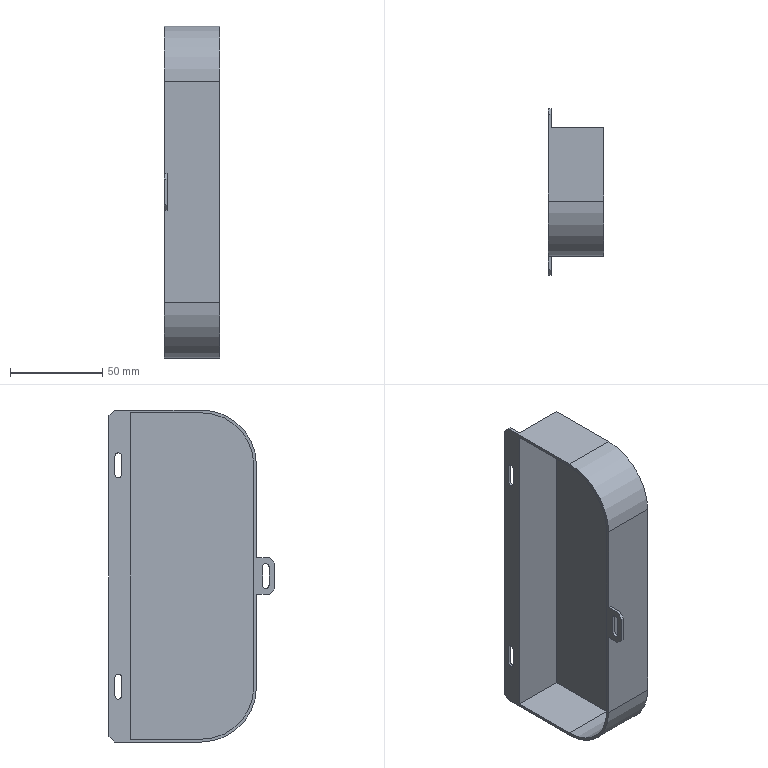Part | SolidWorks | features ICE 3, Chamfer 2, Extrusion 1, Shell 1 | 1 solid | 40 faces | box 30 x 90 x 180 mm | volume 41138 mm3 | plane 27 | cylinder 13 | commonest cylinder face diameters 3.5 x9 57 x2 60 x2
STEP:
#1=CARTESIAN_POINT('',(0.,-67.339,-42.431));
#2=VERTEX_POINT('',#1);
#3=CARTESIAN_POINT('',(0.,-65.589,-40.681));
#4=VERTEX_POINT('',#3);
#5=CARTESIAN_POINT('',(0.,-67.339,-40.681));
#6=DIRECTION('',(1.,0.,0.));
#7=DIRECTION('',(0.,0.,-1.));
#8=AXIS2_PLACEMENT_3D('',#5,#6,#7);
#9=CIRCLE('',#8,1.75);
#10=EDGE_CURVE('',#2,#4,#9,.T.);
#11=ORIENTED_EDGE('',*,*,#10,.F.);
#12=CARTESIAN_POINT('',(1.5,-67.339,-42.431));
#13=VERTEX_POINT('',#12);
#14=CARTESIAN_POINT('',(0.,-67.339,-42.431));
#15=DIRECTION('',(1.,0.,0.));
#16=VECTOR('',#15,1000.);
#17=LINE('',#14,#16);
#18=EDGE_CURVE('',#2,#13,#17,.T.);
#19=ORIENTED_EDGE('',*,*,#18,.T.);
#20=CARTESIAN_POINT('',(1.5,-65.589,-40.681));
#21=VERTEX_POINT('',#20);
#22=CARTESIAN_POINT('',(1.5,-67.339,-40.681));
#23=DIRECTION('',(1.,0.,0.));
#24=DIRECTION('',(0.,0.,-1.));
#25=AXIS2_PLACEMENT_3D('',#22,#23,#24);
#26=CIRCLE('',#25,1.75);
#27=EDGE_CURVE('',#13,#21,#26,.T.);
#28=ORIENTED_EDGE('',*,*,#27,.T.);
#29=CARTESIAN_POINT('',(0.,-65.589,-40.681));
#30=DIRECTION('',(1.,0.,0.));
#31=VECTOR('',#30,1000.);
#32=LINE('',#29,#31);
#33=EDGE_CURVE('',#4,#21,#32,.T.);
#34=ORIENTED_EDGE('',*,*,#33,.F.);
#35=EDGE_LOOP('',(#11,#19,#28,#34));
#36=FACE_OUTER_BOUND('',#35,.T.);
#37=CARTESIAN_POINT('',(0.,-67.339,-40.681));
#38=DIRECTION('',(1.,0.,0.));
#39=DIRECTION('',(0.,0.,-1.));
#40=AXIS2_PLACEMENT_3D('',#37,#38,#39);
#41=CYLINDRICAL_SURFACE('',#40,1.75);
#42=ADVANCED_FACE('',(#36),#41,.F.);
#43=CARTESIAN_POINT('',(0.,12.661,-102.431));
#44=VERTEX_POINT('',#43);
#45=CARTESIAN_POINT('',(0.,14.411,-100.681));
#46=VERTEX_POINT('',#45);
#47=CARTESIAN_POINT('',(0.,12.661,-100.681));
#48=DIRECTION('',(1.,0.,0.));
#49=DIRECTION('',(0.,0.,-1.));
#50=AXIS2_PLACEMENT_3D('',#47,#48,#49);
#51=CIRCLE('',#50,1.75);
#52=EDGE_CURVE('',#44,#46,#51,.T.);
#53=ORIENTED_EDGE('',*,*,#52,.F.);
#54=CARTESIAN_POINT('',(1.5,12.661,-102.431));
#55=VERTEX_POINT('',#54);
#56=CARTESIAN_POINT('',(0.,12.661,-102.431));
#57=DIRECTION('',(1.,0.,0.));
#58=VECTOR('',#57,1000.);
#59=LINE('',#56,#58);
#60=EDGE_CURVE('',#44,#55,#59,.T.);
#61=ORIENTED_EDGE('',*,*,#60,.T.);
#62=CARTESIAN_POINT('',(1.5,14.411,-100.681));
#63=VERTEX_POINT('',#62);
#64=CARTESIAN_POINT('',(1.5,12.661,-100.681));
#65=DIRECTION('',(1.,0.,0.));
#66=DIRECTION('',(0.,0.,-1.));
#67=AXIS2_PLACEMENT_3D('',#64,#65,#66);
#68=CIRCLE('',#67,1.75);
#69=EDGE_CURVE('',#55,#63,#68,.T.);
#70=ORIENTED_EDGE('',*,*,#69,.T.);
#71=CARTESIAN_POINT('',(0.,14.411,-100.681));
#72=DIRECTION('',(1.,0.,0.));
#73=VECTOR('',#72,1000.);
#74=LINE('',#71,#73);
#75=EDGE_CURVE('',#46,#63,#74,.T.);
#76=ORIENTED_EDGE('',*,*,#75,.F.);
#77=EDGE_LOOP('',(#53,#61,#70,#76));
#78=FACE_OUTER_BOUND('',#77,.T.);
#79=CARTESIAN_POINT('',(0.,12.661,-100.681));
#80=DIRECTION('',(1.,0.,0.));
#81=DIRECTION('',(0.,0.,-1.));
#82=AXIS2_PLACEMENT_3D('',#79,#80,#81);
#83=CYLINDRICAL_SURFACE('',#82,1.75);
#84=ADVANCED_FACE('',(#78),#83,.F.);
#85=CARTESIAN_POINT('',(0.,12.661,17.569));
#86=VERTEX_POINT('',#85);
#87=CARTESIAN_POINT('',(0.,14.411,19.319));
#88=VERTEX_POINT('',#87);
#89=CARTESIAN_POINT('',(0.,12.661,19.319));
#90=DIRECTION('',(1.,0.,0.));
#91=DIRECTION('',(0.,0.,-1.));
#92=AXIS2_PLACEMENT_3D('',#89,#90,#91);
#93=CIRCLE('',#92,1.75);
#94=EDGE_CURVE('',#86,#88,#93,.T.);
#95=ORIENTED_EDGE('',*,*,#94,.F.);
#96=CARTESIAN_POINT('',(1.5,12.661,17.569));
#97=VERTEX_POINT('',#96);
#98=CARTESIAN_POINT('',(0.,12.661,17.569));
#99=DIRECTION('',(1.,0.,0.));
#100=VECTOR('',#99,1000.);
#101=LINE('',#98,#100);
#102=EDGE_CURVE('',#86,#97,#101,.T.);
#103=ORIENTED_EDGE('',*,*,#102,.T.);
#104=CARTESIAN_POINT('',(1.5,14.411,19.319));
#105=VERTEX_POINT('',#104);
#106=CARTESIAN_POINT('',(1.5,12.661,19.319));
#107=DIRECTION('',(1.,0.,0.));
#108=DIRECTION('',(0.,0.,-1.));
#109=AXIS2_PLACEMENT_3D('',#106,#107,#108);
#110=CIRCLE('',#109,1.75);
#111=EDGE_CURVE('',#97,#105,#110,.T.);
#112=ORIENTED_EDGE('',*,*,#111,.T.);
#113=CARTESIAN_POINT('',(0.,14.411,19.319));
#114=DIRECTION('',(1.,0.,0.));
#115=VECTOR('',#114,1000.);
#116=LINE('',#113,#115);
#117=EDGE_CURVE('',#88,#105,#116,.T.);
#118=ORIENTED_EDGE('',*,*,#117,.F.);
#119=EDGE_LOOP('',(#95,#103,#112,#118));
#120=FACE_OUTER_BOUND('',#119,.T.);
#121=CARTESIAN_POINT('',(0.,12.661,19.319));
#122=DIRECTION('',(1.,0.,0.));
#123=DIRECTION('',(0.,0.,-1.));
#124=AXIS2_PLACEMENT_3D('',#121,#122,#123);
#125=CYLINDRICAL_SURFACE('',#124,1.75);
#126=ADVANCED_FACE('',(#120),#125,.F.);
#127=CARTESIAN_POINT('',(0.,-62.339,-45.681));
#128=VERTEX_POINT('',#127);
#129=CARTESIAN_POINT('',(1.5,-62.339,-45.681));
#130=VERTEX_POINT('',#129);
#131=CARTESIAN_POINT('',(0.,-62.339,-45.681));
#132=DIRECTION('',(1.,0.,0.));
#133=VECTOR('',#132,1000.);
#134=LINE('',#131,#133);
#135=EDGE_CURVE('',#128,#130,#134,.T.);
#136=ORIENTED_EDGE('',*,*,#135,.F.);
#137=CARTESIAN_POINT('',(0.,-62.339,-95.681));
#138=VERTEX_POINT('',#137);
#139=CARTESIAN_POINT('',(0.,-62.339,24.319));
#140=DIRECTION('',(0.,0.,-1.));
#141=VECTOR('',#140,1000.);
#142=LINE('',#139,#141);
#143=EDGE_CURVE('',#128,#138,#142,.T.);
#144=ORIENTED_EDGE('',*,*,#143,.T.);
#145=CARTESIAN_POINT('',(30.,-62.339,-95.681));
#146=VERTEX_POINT('',#145);
#147=CARTESIAN_POINT('',(30.,-62.339,-95.681));
#148=DIRECTION('',(-1.,0.,0.));
#149=VECTOR('',#148,1000.);
#150=LINE('',#147,#149);
#151=EDGE_CURVE('',#146,#138,#150,.T.);
#152=ORIENTED_EDGE('',*,*,#151,.F.);
#153=CARTESIAN_POINT('',(30.,-62.339,24.319));
#154=VERTEX_POINT('',#153);
#155=CARTESIAN_POINT('',(30.,-62.339,24.319));
#156=DIRECTION('',(0.,0.,-1.));
#157=VECTOR('',#156,1000.);
#158=LINE('',#155,#157);
#159=EDGE_CURVE('',#154,#146,#158,.T.);
#160=ORIENTED_EDGE('',*,*,#159,.F.);
#161=CARTESIAN_POINT('',(0.,-62.339,24.319));
#162=VERTEX_POINT('',#161);
#163=CARTESIAN_POINT('',(30.,-62.339,24.319));
#164=DIRECTION('',(-1.,0.,0.));
#165=VECTOR('',#164,1000.);
#166=LINE('',#163,#165);
#167=EDGE_CURVE('',#154,#162,#166,.T.);
#168=ORIENTED_EDGE('',*,*,#167,.T.);
#169=CARTESIAN_POINT('',(0.,-62.339,-25.681));
#170=VERTEX_POINT('',#169);
#171=CARTESIAN_POINT('',(0.,-62.339,24.319));
#172=DIRECTION('',(0.,0.,-1.));
#173=VECTOR('',#172,1000.);
#174=LINE('',#171,#173);
#175=EDGE_CURVE('',#162,#170,#174,.T.);
#176=ORIENTED_EDGE('',*,*,#175,.T.);
#177=CARTESIAN_POINT('',(1.5,-62.339,-25.681));
#178=VERTEX_POINT('',#177);
#179=CARTESIAN_POINT('',(0.,-62.339,-25.681));
#180=DIRECTION('',(-1.,0.,0.));
#181=VECTOR('',#180,1000.);
#182=LINE('',#179,#181);
#183=EDGE_CURVE('',#178,#170,#182,.T.);
#184=ORIENTED_EDGE('',*,*,#183,.F.);
#185=CARTESIAN_POINT('',(1.5,-62.339,-25.681));
#186=DIRECTION('',(0.,0.,1.));
#187=VECTOR('',#186,1000.);
#188=LINE('',#185,#187);
#189=EDGE_CURVE('',#130,#178,#188,.T.);
#190=ORIENTED_EDGE('',*,*,#189,.F.);
#191=EDGE_LOOP('',(#136,#144,#152,#160,#168,#176,#184,#190));
#192=FACE_OUTER_BOUND('',#191,.T.);
#193=CARTESIAN_POINT('',(30.,-62.339,24.319));
#194=DIRECTION('',(0.,1.,0.));
#195=DIRECTION('',(0.,0.,1.));
#196=AXIS2_PLACEMENT_3D('',#193,#194,#195);
#197=PLANE('',#196);
#198=ADVANCED_FACE('',(#192),#197,.F.);
#199=CARTESIAN_POINT('',(1.5,7.661,54.319));
#200=VERTEX_POINT('',#199);
#201=CARTESIAN_POINT('',(1.5,7.661,-125.681));
#202=VERTEX_POINT('',#201);
#203=CARTESIAN_POINT('',(1.5,7.661,54.319));
#204=DIRECTION('',(0.,0.,-1.));
#205=VECTOR('',#204,1000.);
#206=LINE('',#203,#205);
#207=EDGE_CURVE('',#200,#202,#206,.T.);
#208=ORIENTED_EDGE('',*,*,#207,.F.);
#209=CARTESIAN_POINT('',(30.,7.661,54.319));
#210=VERTEX_POINT('',#209);
#211=CARTESIAN_POINT('',(30.,7.661,54.319));
#212=DIRECTION('',(-1.,0.,0.));
#213=VECTOR('',#212,1000.);
#214=LINE('',#211,#213);
#215=EDGE_CURVE('',#210,#200,#214,.T.);
#216=ORIENTED_EDGE('',*,*,#215,.F.);
#217=CARTESIAN_POINT('',(30.,7.661,-125.681));
#218=VERTEX_POINT('',#217);
#219=CARTESIAN_POINT('',(30.,7.661,54.319));
#220=DIRECTION('',(0.,0.,1.));
#221=VECTOR('',#220,1000.);
#222=LINE('',#219,#221);
#223=EDGE_CURVE('',#218,#210,#222,.T.);
#224=ORIENTED_EDGE('',*,*,#223,.F.);
#225=CARTESIAN_POINT('',(30.,7.661,-125.681));
#226=DIRECTION('',(-1.,0.,0.));
#227=VECTOR('',#226,1000.);
#228=LINE('',#225,#227);
#229=EDGE_CURVE('',#218,#202,#228,.T.);
#230=ORIENTED_EDGE('',*,*,#229,.T.);
#231=EDGE_LOOP('',(#208,#216,#224,#230));
#232=FACE_OUTER_BOUND('',#231,.T.);
#233=CARTESIAN_POINT('',(30.,7.661,54.319));
#234=DIRECTION('',(0.,-1.,0.));
#235=DIRECTION('',(0.,0.,-1.));
#236=AXIS2_PLACEMENT_3D('',#233,#234,#235);
#237=PLANE('',#236);
#238=ADVANCED_FACE('',(#232),#237,.F.);
#239=CARTESIAN_POINT('',(0.,-65.589,-30.681));
#240=VERTEX_POINT('',#239);
#241=CARTESIAN_POINT('',(0.,-69.089,-30.681));
#242=VERTEX_POINT('',#241);
#243=CARTESIAN_POINT('',(0.,-67.339,-30.681));
#244=DIRECTION('',(1.,0.,0.));
#245=DIRECTION('',(0.,0.,-1.));
#246=AXIS2_PLACEMENT_3D('',#243,#244,#245);
#247=CIRCLE('',#246,1.75);
#248=EDGE_CURVE('',#240,#242,#247,.T.);
#249=ORIENTED_EDGE('',*,*,#248,.T.);
#250=CARTESIAN_POINT('',(0.,-69.089,-40.681));
#251=VERTEX_POINT('',#250);
#252=CARTESIAN_POINT('',(0.,-69.089,-30.681));
#253=DIRECTION('',(0.,0.,-1.));
#254=VECTOR('',#253,1000.);
#255=LINE('',#252,#254);
#256=EDGE_CURVE('',#242,#251,#255,.T.);
#257=ORIENTED_EDGE('',*,*,#256,.T.);
#258=CARTESIAN_POINT('',(0.,-67.339,-40.681));
#259=DIRECTION('',(1.,0.,0.));
#260=DIRECTION('',(0.,0.,-1.));
#261=AXIS2_PLACEMENT_3D('',#258,#259,#260);
#262=CIRCLE('',#261,1.75);
#263=EDGE_CURVE('',#251,#2,#262,.T.);
#264=ORIENTED_EDGE('',*,*,#263,.T.);
#265=ORIENTED_EDGE('',*,*,#10,.T.);
#266=CARTESIAN_POINT('',(0.,-65.589,-30.681));
#267=DIRECTION('',(0.,0.,1.));
#268=VECTOR('',#267,1000.);
#269=LINE('',#266,#268);
#270=EDGE_CURVE('',#4,#240,#269,.T.);
#271=ORIENTED_EDGE('',*,*,#270,.T.);
#272=EDGE_LOOP('',(#249,#257,#264,#265,#271));
#273=FACE_BOUND('',#272,.T.);
#274=CARTESIAN_POINT('',(0.,14.411,-90.681));
#275=VERTEX_POINT('',#274);
#276=CARTESIAN_POINT('',(0.,10.911,-90.681));
#277=VERTEX_POINT('',#276);
#278=CARTESIAN_POINT('',(0.,12.661,-90.681));
#279=DIRECTION('',(1.,0.,0.));
#280=DIRECTION('',(0.,0.,-1.));
#281=AXIS2_PLACEMENT_3D('',#278,#279,#280);
#282=CIRCLE('',#281,1.75);
#283=EDGE_CURVE('',#275,#277,#282,.T.);
#284=ORIENTED_EDGE('',*,*,#283,.T.);
#285=CARTESIAN_POINT('',(0.,10.911,-100.681));
#286=VERTEX_POINT('',#285);
#287=CARTESIAN_POINT('',(0.,10.911,-90.681));
#288=DIRECTION('',(0.,0.,-1.));
#289=VECTOR('',#288,1000.);
#290=LINE('',#287,#289);
#291=EDGE_CURVE('',#277,#286,#290,.T.);
#292=ORIENTED_EDGE('',*,*,#291,.T.);
#293=CARTESIAN_POINT('',(0.,12.661,-100.681));
#294=DIRECTION('',(1.,0.,0.));
#295=DIRECTION('',(0.,0.,-1.));
#296=AXIS2_PLACEMENT_3D('',#293,#294,#295);
#297=CIRCLE('',#296,1.75);
#298=EDGE_CURVE('',#286,#44,#297,.T.);
#299=ORIENTED_EDGE('',*,*,#298,.T.);
#300=ORIENTED_EDGE('',*,*,#52,.T.);
#301=CARTESIAN_POINT('',(0.,14.411,-90.681));
#302=DIRECTION('',(0.,0.,1.));
#303=VECTOR('',#302,1000.);
#304=LINE('',#301,#303);
#305=EDGE_CURVE('',#46,#275,#304,.T.);
#306=ORIENTED_EDGE('',*,*,#305,.T.);
#307=EDGE_LOOP('',(#284,#292,#299,#300,#306));
#308=FACE_BOUND('',#307,.T.);
#309=CARTESIAN_POINT('',(0.,14.411,29.319));
#310=VERTEX_POINT('',#309);
#311=CARTESIAN_POINT('',(0.,10.911,29.319));
#312=VERTEX_POINT('',#311);
#313=CARTESIAN_POINT('',(0.,12.661,29.319));
#314=DIRECTION('',(1.,0.,0.));
#315=DIRECTION('',(0.,0.,-1.));
#316=AXIS2_PLACEMENT_3D('',#313,#314,#315);
#317=CIRCLE('',#316,1.75);
#318=EDGE_CURVE('',#310,#312,#317,.T.);
#319=ORIENTED_EDGE('',*,*,#318,.T.);
#320=CARTESIAN_POINT('',(0.,10.911,19.319));
#321=VERTEX_POINT('',#320);
#322=CARTESIAN_POINT('',(0.,10.911,29.319));
#323=DIRECTION('',(0.,0.,-1.));
#324=VECTOR('',#323,1000.);
#325=LINE('',#322,#324);
#326=EDGE_CURVE('',#312,#321,#325,.T.);
#327=ORIENTED_EDGE('',*,*,#326,.T.);
#328=CARTESIAN_POINT('',(0.,12.661,19.319));
#329=DIRECTION('',(1.,0.,0.));
#330=DIRECTION('',(0.,0.,-1.));
#331=AXIS2_PLACEMENT_3D('',#328,#329,#330);
#332=CIRCLE('',#331,1.75);
#333=EDGE_CURVE('',#321,#86,#332,.T.);
#334=ORIENTED_EDGE('',*,*,#333,.T.);
#335=ORIENTED_EDGE('',*,*,#94,.T.);
#336=CARTESIAN_POINT('',(0.,14.411,29.319));
#337=DIRECTION('',(0.,0.,1.));
#338=VECTOR('',#337,1000.);
#339=LINE('',#336,#338);
#340=EDGE_CURVE('',#88,#310,#339,.T.);
#341=ORIENTED_EDGE('',*,*,#340,.T.);
#342=EDGE_LOOP('',(#319,#327,#334,#335,#341));
#343=FACE_BOUND('',#342,.T.);
#344=CARTESIAN_POINT('',(0.,-72.339,-28.681));
#345=VERTEX_POINT('',#344);
#346=CARTESIAN_POINT('',(0.,-72.339,-42.681));
#347=VERTEX_POINT('',#346);
#348=CARTESIAN_POINT('',(0.,-72.339,-25.681));
#349=DIRECTION('',(0.,0.,-1.));
#350=VECTOR('',#349,1000.);
#351=LINE('',#348,#350);
#352=EDGE_CURVE('',#345,#347,#351,.T.);
#353=ORIENTED_EDGE('',*,*,#352,.F.);
#354=CARTESIAN_POINT('',(0.,-69.339,-25.681));
#355=VERTEX_POINT('',#354);
#356=CARTESIAN_POINT('',(0.,-25.839,17.819));
#357=DIRECTION('',(0.,0.7071,0.7071));
#358=VECTOR('',#357,1000.);
#359=LINE('',#356,#358);
#360=EDGE_CURVE('',#345,#355,#359,.T.);
#361=ORIENTED_EDGE('',*,*,#360,.T.);
#362=CARTESIAN_POINT('',(0.,-72.339,-25.681));
#363=DIRECTION('',(0.,1.,0.));
#364=VECTOR('',#363,1000.);
#365=LINE('',#362,#364);
#366=EDGE_CURVE('',#355,#170,#365,.T.);
#367=ORIENTED_EDGE('',*,*,#366,.T.);
#368=ORIENTED_EDGE('',*,*,#175,.F.);
#369=CARTESIAN_POINT('',(0.,-32.339,54.319));
#370=VERTEX_POINT('',#369);
#371=CARTESIAN_POINT('',(0.,-32.339,24.319));
#372=DIRECTION('',(1.,0.,0.));
#373=DIRECTION('',(0.,0.,1.));
#374=AXIS2_PLACEMENT_3D('',#371,#372,#373);
#375=CIRCLE('',#374,30.);
#376=EDGE_CURVE('',#370,#162,#375,.T.);
#377=ORIENTED_EDGE('',*,*,#376,.F.);
#378=CARTESIAN_POINT('',(0.,14.661,54.319));
#379=VERTEX_POINT('',#378);
#380=CARTESIAN_POINT('',(0.,7.661,54.319));
#381=DIRECTION('',(0.,-1.,0.));
#382=VECTOR('',#381,1000.);
#383=LINE('',#380,#382);
#384=EDGE_CURVE('',#379,#370,#383,.T.);
#385=ORIENTED_EDGE('',*,*,#384,.F.);
#386=CARTESIAN_POINT('',(0.,17.661,51.319));
#387=VERTEX_POINT('',#386);
#388=CARTESIAN_POINT('',(0.,6.161,62.819));
#389=DIRECTION('',(0.,0.7071,-0.7071));
#390=VECTOR('',#389,1000.);
#391=LINE('',#388,#390);
#392=EDGE_CURVE('',#379,#387,#391,.T.);
#393=ORIENTED_EDGE('',*,*,#392,.T.);
#394=CARTESIAN_POINT('',(0.,17.661,-122.681));
#395=VERTEX_POINT('',#394);
#396=CARTESIAN_POINT('',(0.,17.661,54.319));
#397=DIRECTION('',(0.,0.,1.));
#398=VECTOR('',#397,1000.);
#399=LINE('',#396,#398);
#400=EDGE_CURVE('',#395,#387,#399,.T.);
#401=ORIENTED_EDGE('',*,*,#400,.F.);
#402=CARTESIAN_POINT('',(0.,14.661,-125.681));
#403=VERTEX_POINT('',#402);
#404=CARTESIAN_POINT('',(0.,66.161,-74.181));
#405=DIRECTION('',(0.,-0.7071,-0.7071));
#406=VECTOR('',#405,1000.);
#407=LINE('',#404,#406);
#408=EDGE_CURVE('',#395,#403,#407,.T.);
#409=ORIENTED_EDGE('',*,*,#408,.T.);
#410=CARTESIAN_POINT('',(0.,-32.339,-125.681));
#411=VERTEX_POINT('',#410);
#412=CARTESIAN_POINT('',(0.,7.661,-125.681));
#413=DIRECTION('',(0.,1.,0.));
#414=VECTOR('',#413,1000.);
#415=LINE('',#412,#414);
#416=EDGE_CURVE('',#411,#403,#415,.T.);
#417=ORIENTED_EDGE('',*,*,#416,.F.);
#418=CARTESIAN_POINT('',(0.,-32.339,-95.681));
#419=DIRECTION('',(1.,0.,0.));
#420=DIRECTION('',(0.,0.,-1.));
#421=AXIS2_PLACEMENT_3D('',#418,#419,#420);
#422=CIRCLE('',#421,30.);
#423=EDGE_CURVE('',#138,#411,#422,.T.);
#424=ORIENTED_EDGE('',*,*,#423,.F.);
#425=ORIENTED_EDGE('',*,*,#143,.F.);
#426=CARTESIAN_POINT('',(0.,-69.339,-45.681));
#427=VERTEX_POINT('',#426);
#428=CARTESIAN_POINT('',(0.,-72.339,-45.681));
#429=DIRECTION('',(0.,1.,0.));
#430=VECTOR('',#429,1000.);
#431=LINE('',#428,#430);
#432=EDGE_CURVE('',#427,#128,#431,.T.);
#433=ORIENTED_EDGE('',*,*,#432,.F.);
#434=CARTESIAN_POINT('',(0.,-85.839,-29.181));
#435=DIRECTION('',(0.,-0.7071,0.7071));
#436=VECTOR('',#435,1000.);
#437=LINE('',#434,#436);
#438=EDGE_CURVE('',#427,#347,#437,.T.);
#439=ORIENTED_EDGE('',*,*,#438,.T.);
#440=EDGE_LOOP('',(#353,#361,#367,#368,#377,#385,#393,#401,#409,#417,#424,#425,#433,#439));
#441=FACE_OUTER_BOUND('',#440,.T.);
#442=CARTESIAN_POINT('',(0.,6.161,-124.181));
#443=VERTEX_POINT('',#442);
#444=CARTESIAN_POINT('',(0.,6.161,52.819));
#445=VERTEX_POINT('',#444);
#446=CARTESIAN_POINT('',(0.,6.161,24.319));
#447=DIRECTION('',(0.,0.,1.));
#448=VECTOR('',#447,1000.);
#449=LINE('',#446,#448);
#450=EDGE_CURVE('',#443,#445,#449,.T.);
#451=ORIENTED_EDGE('',*,*,#450,.T.);
#452=CARTESIAN_POINT('',(0.,-32.339,52.819));
#453=VERTEX_POINT('',#452);
#454=CARTESIAN_POINT('',(0.,-32.339,52.819));
#455=DIRECTION('',(0.,-1.,0.));
#456=VECTOR('',#455,1000.);
#457=LINE('',#454,#456);
#458=EDGE_CURVE('',#445,#453,#457,.T.);
#459=ORIENTED_EDGE('',*,*,#458,.T.);
#460=CARTESIAN_POINT('',(0.,-60.839,24.319));
#461=VERTEX_POINT('',#460);
#462=CARTESIAN_POINT('',(0.,-32.339,24.319));
#463=DIRECTION('',(1.,0.,0.));
#464=DIRECTION('',(0.,0.,1.));
#465=AXIS2_PLACEMENT_3D('',#462,#463,#464);
#466=CIRCLE('',#465,28.5);
#467=EDGE_CURVE('',#453,#461,#466,.T.);
#468=ORIENTED_EDGE('',*,*,#467,.T.);
#469=CARTESIAN_POINT('',(0.,-60.839,-95.681));
#470=VERTEX_POINT('',#469);
#471=CARTESIAN_POINT('',(0.,-60.839,24.319));
#472=DIRECTION('',(0.,0.,-1.));
#473=VECTOR('',#472,1000.);
#474=LINE('',#471,#473);
#475=EDGE_CURVE('',#461,#470,#474,.T.);
#476=ORIENTED_EDGE('',*,*,#475,.T.);
#477=CARTESIAN_POINT('',(0.,-32.339,-124.181));
#478=VERTEX_POINT('',#477);
#479=CARTESIAN_POINT('',(0.,-32.339,-95.681));
#480=DIRECTION('',(1.,0.,0.));
#481=DIRECTION('',(0.,0.,1.));
#482=AXIS2_PLACEMENT_3D('',#479,#480,#481);
#483=CIRCLE('',#482,28.5);
#484=EDGE_CURVE('',#470,#478,#483,.T.);
#485=ORIENTED_EDGE('',*,*,#484,.T.);
#486=CARTESIAN_POINT('',(0.,-32.339,-124.181));
#487=DIRECTION('',(0.,1.,0.));
#488=VECTOR('',#487,1000.);
#489=LINE('',#486,#488);
#490=EDGE_CURVE('',#478,#443,#489,.T.);
#491=ORIENTED_EDGE('',*,*,#490,.T.);
#492=EDGE_LOOP('',(#451,#459,#468,#476,#485,#491));
#493=FACE_BOUND('',#492,.T.);
#494=CARTESIAN_POINT('',(0.,-32.339,24.319));
#495=DIRECTION('',(-1.,0.,0.));
#496=DIRECTION('',(0.,0.,1.));
#497=AXIS2_PLACEMENT_3D('',#494,#495,#496);
#498=PLANE('',#497);
#499=ADVANCED_FACE('',(#273,#308,#343,#441,#493),#498,.T.);
#500=CARTESIAN_POINT('',(1.5,14.661,54.319));
#501=VERTEX_POINT('',#500);
#502=CARTESIAN_POINT('',(1.5,17.661,54.319));
#503=DIRECTION('',(0.,-1.,0.));
#504=VECTOR('',#503,1000.);
#505=LINE('',#502,#504);
#506=EDGE_CURVE('',#501,#200,#505,.T.);
#507=ORIENTED_EDGE('',*,*,#506,.F.);
#508=CARTESIAN_POINT('',(30.,14.661,54.319));
#509=DIRECTION('',(-1.,0.,0.));
#510=VECTOR('',#509,1000.);
#511=LINE('',#508,#510);
#512=EDGE_CURVE('',#501,#379,#511,.T.);
#513=ORIENTED_EDGE('',*,*,#512,.T.);
#514=ORIENTED_EDGE('',*,*,#384,.T.);
#515=CARTESIAN_POINT('',(30.,-32.339,54.319));
#516=VERTEX_POINT('',#515);
#517=CARTESIAN_POINT('',(30.,-32.339,54.319));
#518=DIRECTION('',(-1.,0.,0.));
#519=VECTOR('',#518,1000.);
#520=LINE('',#517,#519);
#521=EDGE_CURVE('',#516,#370,#520,.T.);
#522=ORIENTED_EDGE('',*,*,#521,.F.);
#523=CARTESIAN_POINT('',(30.,7.661,54.319));
#524=DIRECTION('',(0.,-1.,0.));
#525=VECTOR('',#524,1000.);
#526=LINE('',#523,#525);
#527=EDGE_CURVE('',#210,#516,#526,.T.);
#528=ORIENTED_EDGE('',*,*,#527,.F.);
#529=ORIENTED_EDGE('',*,*,#215,.T.);
#530=EDGE_LOOP('',(#507,#513,#514,#522,#528,#529));
#531=FACE_OUTER_BOUND('',#530,.T.);
#532=CARTESIAN_POINT('',(30.,7.661,54.319));
#533=DIRECTION('',(0.,0.,-1.));
#534=DIRECTION('',(0.,1.,0.));
#535=AXIS2_PLACEMENT_3D('',#532,#533,#534);
#536=PLANE('',#535);
#537=ADVANCED_FACE('',(#531),#536,.F.);
#538=ORIENTED_EDGE('',*,*,#376,.T.);
#539=ORIENTED_EDGE('',*,*,#167,.F.);
#540=CARTESIAN_POINT('',(30.,-32.339,24.319));
#541=DIRECTION('',(1.,0.,0.));
#542=DIRECTION('',(0.,0.,1.));
#543=AXIS2_PLACEMENT_3D('',#540,#541,#542);
#544=CIRCLE('',#543,30.);
#545=EDGE_CURVE('',#516,#154,#544,.T.);
#546=ORIENTED_EDGE('',*,*,#545,.F.);
#547=ORIENTED_EDGE('',*,*,#521,.T.);
#548=EDGE_LOOP('',(#538,#539,#546,#547));
#549=FACE_OUTER_BOUND('',#548,.T.);
#550=CARTESIAN_POINT('',(30.,-32.339,24.319));
#551=DIRECTION('',(-1.,0.,0.));
#552=DIRECTION('',(0.,0.,1.));
#553=AXIS2_PLACEMENT_3D('',#550,#551,#552);
#554=CYLINDRICAL_SURFACE('',#553,30.);
#555=ADVANCED_FACE('',(#549),#554,.T.);
#556=ORIENTED_EDGE('',*,*,#423,.T.);
#557=CARTESIAN_POINT('',(30.,-32.339,-125.681));
#558=VERTEX_POINT('',#557);
#559=CARTESIAN_POINT('',(30.,-32.339,-125.681));
#560=DIRECTION('',(-1.,0.,0.));
#561=VECTOR('',#560,1000.);
#562=LINE('',#559,#561);
#563=EDGE_CURVE('',#558,#411,#562,.T.);
#564=ORIENTED_EDGE('',*,*,#563,.F.);
#565=CARTESIAN_POINT('',(30.,-32.339,-95.681));
#566=DIRECTION('',(1.,0.,0.));
#567=DIRECTION('',(0.,0.,-1.));
#568=AXIS2_PLACEMENT_3D('',#565,#566,#567);
#569=CIRCLE('',#568,30.);
#570=EDGE_CURVE('',#146,#558,#569,.T.);
#571=ORIENTED_EDGE('',*,*,#570,.F.);
#572=ORIENTED_EDGE('',*,*,#151,.T.);
#573=EDGE_LOOP('',(#556,#564,#571,#572));
#574=FACE_OUTER_BOUND('',#573,.T.);
#575=CARTESIAN_POINT('',(30.,-32.339,-95.681));
#576=DIRECTION('',(-1.,0.,0.));
#577=DIRECTION('',(0.,0.,1.));
#578=AXIS2_PLACEMENT_3D('',#575,#576,#577);
#579=CYLINDRICAL_SURFACE('',#578,30.);
#580=ADVANCED_FACE('',(#574),#579,.T.);
#581=ORIENTED_EDGE('',*,*,#416,.T.);
#582=CARTESIAN_POINT('',(1.5,14.661,-125.681));
#583=VERTEX_POINT('',#582);
#584=CARTESIAN_POINT('',(30.,14.661,-125.681));
#585=DIRECTION('',(1.,0.,0.));
#586=VECTOR('',#585,1000.);
#587=LINE('',#584,#586);
#588=EDGE_CURVE('',#403,#583,#587,.T.);
#589=ORIENTED_EDGE('',*,*,#588,.T.);
#590=CARTESIAN_POINT('',(1.5,17.661,-125.681));
#591=DIRECTION('',(0.,-1.,0.));
#592=VECTOR('',#591,1000.);
#593=LINE('',#590,#592);
#594=EDGE_CURVE('',#583,#202,#593,.T.);
#595=ORIENTED_EDGE('',*,*,#594,.T.);
#596=ORIENTED_EDGE('',*,*,#229,.F.);
#597=CARTESIAN_POINT('',(30.,7.661,-125.681));
#598=DIRECTION('',(0.,1.,0.));
#599=VECTOR('',#598,1000.);
#600=LINE('',#597,#599);
#601=EDGE_CURVE('',#558,#218,#600,.T.);
#602=ORIENTED_EDGE('',*,*,#601,.F.);
#603=ORIENTED_EDGE('',*,*,#563,.T.);
#604=EDGE_LOOP('',(#581,#589,#595,#596,#602,#603));
#605=FACE_OUTER_BOUND('',#604,.T.);
#606=CARTESIAN_POINT('',(30.,7.661,-125.681));
#607=DIRECTION('',(0.,0.,1.));
#608=DIRECTION('',(1.,0.,0.));
#609=AXIS2_PLACEMENT_3D('',#606,#607,#608);
#610=PLANE('',#609);
#611=ADVANCED_FACE('',(#605),#610,.F.);
#612=ORIENTED_EDGE('',*,*,#527,.T.);
#613=ORIENTED_EDGE('',*,*,#545,.T.);
#614=ORIENTED_EDGE('',*,*,#159,.T.);
#615=ORIENTED_EDGE('',*,*,#570,.T.);
#616=ORIENTED_EDGE('',*,*,#601,.T.);
#617=ORIENTED_EDGE('',*,*,#223,.T.);
#618=EDGE_LOOP('',(#612,#613,#614,#615,#616,#617));
#619=FACE_OUTER_BOUND('',#618,.T.);
#620=CARTESIAN_POINT('',(30.,-32.339,24.319));
#621=DIRECTION('',(-1.,0.,0.));
#622=DIRECTION('',(0.,0.,1.));
#623=AXIS2_PLACEMENT_3D('',#620,#621,#622);
#624=PLANE('',#623);
#625=ADVANCED_FACE('',(#619),#624,.F.);
#626=ORIENTED_EDGE('',*,*,#458,.F.);
#627=CARTESIAN_POINT('',(28.5,6.161,52.819));
#628=VERTEX_POINT('',#627);
#629=CARTESIAN_POINT('',(30.,6.161,52.819));
#630=DIRECTION('',(-1.,0.,0.));
#631=VECTOR('',#630,1000.);
#632=LINE('',#629,#631);
#633=EDGE_CURVE('',#628,#445,#632,.T.);
#634=ORIENTED_EDGE('',*,*,#633,.F.);
#635=CARTESIAN_POINT('',(28.5,-32.339,52.819));
#636=VERTEX_POINT('',#635);
#637=CARTESIAN_POINT('',(28.5,-32.339,52.819));
#638=DIRECTION('',(0.,-1.,0.));
#639=VECTOR('',#638,1000.);
#640=LINE('',#637,#639);
#641=EDGE_CURVE('',#628,#636,#640,.T.);
#642=ORIENTED_EDGE('',*,*,#641,.T.);
#643=CARTESIAN_POINT('',(30.,-32.339,52.819));
#644=DIRECTION('',(-1.,0.,0.));
#645=VECTOR('',#644,1000.);
#646=LINE('',#643,#645);
#647=EDGE_CURVE('',#636,#453,#646,.T.);
#648=ORIENTED_EDGE('',*,*,#647,.T.);
#649=EDGE_LOOP('',(#626,#634,#642,#648));
#650=FACE_OUTER_BOUND('',#649,.T.);
#651=CARTESIAN_POINT('',(30.,7.661,52.819));
#652=DIRECTION('',(0.,0.,-1.));
#653=DIRECTION('',(0.,1.,0.));
#654=AXIS2_PLACEMENT_3D('',#651,#652,#653);
#655=PLANE('',#654);
#656=ADVANCED_FACE('',(#650),#655,.T.);
#657=ORIENTED_EDGE('',*,*,#467,.F.);
#658=ORIENTED_EDGE('',*,*,#647,.F.);
#659=CARTESIAN_POINT('',(28.5,-60.839,24.319));
#660=VERTEX_POINT('',#659);
#661=CARTESIAN_POINT('',(28.5,-32.339,24.319));
#662=DIRECTION('',(1.,0.,0.));
#663=DIRECTION('',(0.,0.,1.));
#664=AXIS2_PLACEMENT_3D('',#661,#662,#663);
#665=CIRCLE('',#664,28.5);
#666=EDGE_CURVE('',#636,#660,#665,.T.);
#667=ORIENTED_EDGE('',*,*,#666,.T.);
#668=CARTESIAN_POINT('',(30.,-60.839,24.319));
#669=DIRECTION('',(-1.,0.,0.));
#670=VECTOR('',#669,1000.);
#671=LINE('',#668,#670);
#672=EDGE_CURVE('',#660,#461,#671,.T.);
#673=ORIENTED_EDGE('',*,*,#672,.T.);
#674=EDGE_LOOP('',(#657,#658,#667,#673));
#675=FACE_OUTER_BOUND('',#674,.T.);
#676=CARTESIAN_POINT('',(30.,-32.339,24.319));
#677=DIRECTION('',(-1.,0.,0.));
#678=DIRECTION('',(0.,0.,1.));
#679=AXIS2_PLACEMENT_3D('',#676,#677,#678);
#680=CYLINDRICAL_SURFACE('',#679,28.5);
#681=ADVANCED_FACE('',(#675),#680,.F.);
#682=ORIENTED_EDGE('',*,*,#475,.F.);
#683=ORIENTED_EDGE('',*,*,#672,.F.);
#684=CARTESIAN_POINT('',(28.5,-60.839,-95.681));
#685=VERTEX_POINT('',#684);
#686=CARTESIAN_POINT('',(28.5,-60.839,24.319));
#687=DIRECTION('',(0.,0.,-1.));
#688=VECTOR('',#687,1000.);
#689=LINE('',#686,#688);
#690=EDGE_CURVE('',#660,#685,#689,.T.);
#691=ORIENTED_EDGE('',*,*,#690,.T.);
#692=CARTESIAN_POINT('',(30.,-60.839,-95.681));
#693=DIRECTION('',(-1.,0.,0.));
#694=VECTOR('',#693,1000.);
#695=LINE('',#692,#694);
#696=EDGE_CURVE('',#685,#470,#695,.T.);
#697=ORIENTED_EDGE('',*,*,#696,.T.);
#698=EDGE_LOOP('',(#682,#683,#691,#697));
#699=FACE_OUTER_BOUND('',#698,.T.);
#700=CARTESIAN_POINT('',(30.,-60.839,24.319));
#701=DIRECTION('',(0.,1.,0.));
#702=DIRECTION('',(0.,0.,1.));
#703=AXIS2_PLACEMENT_3D('',#700,#701,#702);
#704=PLANE('',#703);
#705=ADVANCED_FACE('',(#699),#704,.T.);
#706=ORIENTED_EDGE('',*,*,#484,.F.);
#707=ORIENTED_EDGE('',*,*,#696,.F.);
#708=CARTESIAN_POINT('',(28.5,-32.339,-124.181));
#709=VERTEX_POINT('',#708);
#710=CARTESIAN_POINT('',(28.5,-32.339,-95.681));
#711=DIRECTION('',(1.,0.,0.));
#712=DIRECTION('',(0.,0.,1.));
#713=AXIS2_PLACEMENT_3D('',#710,#711,#712);
#714=CIRCLE('',#713,28.5);
#715=EDGE_CURVE('',#685,#709,#714,.T.);
#716=ORIENTED_EDGE('',*,*,#715,.T.);
#717=CARTESIAN_POINT('',(30.,-32.339,-124.181));
#718=DIRECTION('',(-1.,0.,0.));
#719=VECTOR('',#718,1000.);
#720=LINE('',#717,#719);
#721=EDGE_CURVE('',#709,#478,#720,.T.);
#722=ORIENTED_EDGE('',*,*,#721,.T.);
#723=EDGE_LOOP('',(#706,#707,#716,#722));
#724=FACE_OUTER_BOUND('',#723,.T.);
#725=CARTESIAN_POINT('',(30.,-32.339,-95.681));
#726=DIRECTION('',(-1.,0.,0.));
#727=DIRECTION('',(0.,0.,1.));
#728=AXIS2_PLACEMENT_3D('',#725,#726,#727);
#729=CYLINDRICAL_SURFACE('',#728,28.5);
#730=ADVANCED_FACE('',(#724),#729,.F.);
#731=ORIENTED_EDGE('',*,*,#490,.F.);
#732=ORIENTED_EDGE('',*,*,#721,.F.);
#733=CARTESIAN_POINT('',(28.5,6.161,-124.181));
#734=VERTEX_POINT('',#733);
#735=CARTESIAN_POINT('',(28.5,-32.339,-124.181));
#736=DIRECTION('',(0.,1.,0.));
#737=VECTOR('',#736,1000.);
#738=LINE('',#735,#737);
#739=EDGE_CURVE('',#709,#734,#738,.T.);
#740=ORIENTED_EDGE('',*,*,#739,.T.);
#741=CARTESIAN_POINT('',(30.,6.161,-124.181));
#742=DIRECTION('',(-1.,0.,0.));
#743=VECTOR('',#742,1000.);
#744=LINE('',#741,#743);
#745=EDGE_CURVE('',#734,#443,#744,.T.);
#746=ORIENTED_EDGE('',*,*,#745,.T.);
#747=EDGE_LOOP('',(#731,#732,#740,#746));
#748=FACE_OUTER_BOUND('',#747,.T.);
#749=CARTESIAN_POINT('',(30.,7.661,-124.181));
#750=DIRECTION('',(0.,0.,1.));
#751=DIRECTION('',(1.,0.,0.));
#752=AXIS2_PLACEMENT_3D('',#749,#750,#751);
#753=PLANE('',#752);
#754=ADVANCED_FACE('',(#748),#753,.T.);
#755=ORIENTED_EDGE('',*,*,#450,.F.);
#756=ORIENTED_EDGE('',*,*,#745,.F.);
#757=CARTESIAN_POINT('',(28.5,6.161,24.319));
#758=DIRECTION('',(0.,0.,1.));
#759=VECTOR('',#758,1000.);
#760=LINE('',#757,#759);
#761=EDGE_CURVE('',#734,#628,#760,.T.);
#762=ORIENTED_EDGE('',*,*,#761,.T.);
#763=ORIENTED_EDGE('',*,*,#633,.T.);
#764=EDGE_LOOP('',(#755,#756,#762,#763));
#765=FACE_OUTER_BOUND('',#764,.T.);
#766=CARTESIAN_POINT('',(30.,6.161,54.319));
#767=DIRECTION('',(0.,-1.,0.));
#768=DIRECTION('',(0.,0.,-1.));
#769=AXIS2_PLACEMENT_3D('',#766,#767,#768);
#770=PLANE('',#769);
#771=ADVANCED_FACE('',(#765),#770,.T.);
#772=ORIENTED_EDGE('',*,*,#641,.F.);
#773=ORIENTED_EDGE('',*,*,#761,.F.);
#774=ORIENTED_EDGE('',*,*,#739,.F.);
#775=ORIENTED_EDGE('',*,*,#715,.F.);
#776=ORIENTED_EDGE('',*,*,#690,.F.);
#777=ORIENTED_EDGE('',*,*,#666,.F.);
#778=EDGE_LOOP('',(#772,#773,#774,#775,#776,#777));
#779=FACE_OUTER_BOUND('',#778,.T.);
#780=CARTESIAN_POINT('',(28.5,-32.339,24.319));
#781=DIRECTION('',(-1.,0.,0.));
#782=DIRECTION('',(0.,0.,1.));
#783=AXIS2_PLACEMENT_3D('',#780,#781,#782);
#784=PLANE('',#783);
#785=ADVANCED_FACE('',(#779),#784,.T.);
#786=CARTESIAN_POINT('',(1.5,10.911,-90.681));
#787=VERTEX_POINT('',#786);
#788=CARTESIAN_POINT('',(1.5,10.911,-100.681));
#789=VERTEX_POINT('',#788);
#790=CARTESIAN_POINT('',(1.5,10.911,-90.681));
#791=DIRECTION('',(0.,0.,-1.));
#792=VECTOR('',#791,1000.);
#793=LINE('',#790,#792);
#794=EDGE_CURVE('',#787,#789,#793,.T.);
#795=ORIENTED_EDGE('',*,*,#794,.F.);
#796=CARTESIAN_POINT('',(1.5,14.411,-90.681));
#797=VERTEX_POINT('',#796);
#798=CARTESIAN_POINT('',(1.5,12.661,-90.681));
#799=DIRECTION('',(1.,0.,0.));
#800=DIRECTION('',(0.,0.,-1.));
#801=AXIS2_PLACEMENT_3D('',#798,#799,#800);
#802=CIRCLE('',#801,1.75);
#803=EDGE_CURVE('',#797,#787,#802,.T.);
#804=ORIENTED_EDGE('',*,*,#803,.F.);
#805=CARTESIAN_POINT('',(1.5,14.411,-90.681));
#806=DIRECTION('',(0.,0.,1.));
#807=VECTOR('',#806,1000.);
#808=LINE('',#805,#807);
#809=EDGE_CURVE('',#63,#797,#808,.T.);
#810=ORIENTED_EDGE('',*,*,#809,.F.);
#811=ORIENTED_EDGE('',*,*,#69,.F.);
#812=CARTESIAN_POINT('',(1.5,12.661,-100.681));
#813=DIRECTION('',(1.,0.,0.));
#814=DIRECTION('',(0.,0.,-1.));
#815=AXIS2_PLACEMENT_3D('',#812,#813,#814);
#816=CIRCLE('',#815,1.75);
#817=EDGE_CURVE('',#789,#55,#816,.T.);
#818=ORIENTED_EDGE('',*,*,#817,.F.);
#819=EDGE_LOOP('',(#795,#804,#810,#811,#818));
#820=FACE_BOUND('',#819,.T.);
#821=CARTESIAN_POINT('',(1.5,10.911,29.319));
#822=VERTEX_POINT('',#821);
#823=CARTESIAN_POINT('',(1.5,10.911,19.319));
#824=VERTEX_POINT('',#823);
#825=CARTESIAN_POINT('',(1.5,10.911,29.319));
#826=DIRECTION('',(0.,0.,-1.));
#827=VECTOR('',#826,1000.);
#828=LINE('',#825,#827);
#829=EDGE_CURVE('',#822,#824,#828,.T.);
#830=ORIENTED_EDGE('',*,*,#829,.F.);
#831=CARTESIAN_POINT('',(1.5,14.411,29.319));
#832=VERTEX_POINT('',#831);
#833=CARTESIAN_POINT('',(1.5,12.661,29.319));
#834=DIRECTION('',(1.,0.,0.));
#835=DIRECTION('',(0.,0.,-1.));
#836=AXIS2_PLACEMENT_3D('',#833,#834,#835);
#837=CIRCLE('',#836,1.75);
#838=EDGE_CURVE('',#832,#822,#837,.T.);
#839=ORIENTED_EDGE('',*,*,#838,.F.);
#840=CARTESIAN_POINT('',(1.5,14.411,29.319));
#841=DIRECTION('',(0.,0.,1.));
#842=VECTOR('',#841,1000.);
#843=LINE('',#840,#842);
#844=EDGE_CURVE('',#105,#832,#843,.T.);
#845=ORIENTED_EDGE('',*,*,#844,.F.);
#846=ORIENTED_EDGE('',*,*,#111,.F.);
#847=CARTESIAN_POINT('',(1.5,12.661,19.319));
#848=DIRECTION('',(1.,0.,0.));
#849=DIRECTION('',(0.,0.,-1.));
#850=AXIS2_PLACEMENT_3D('',#847,#848,#849);
#851=CIRCLE('',#850,1.75);
#852=EDGE_CURVE('',#824,#97,#851,.T.);
#853=ORIENTED_EDGE('',*,*,#852,.F.);
#854=EDGE_LOOP('',(#830,#839,#845,#846,#853));
#855=FACE_BOUND('',#854,.T.);
#856=ORIENTED_EDGE('',*,*,#594,.F.);
#857=CARTESIAN_POINT('',(1.5,17.661,-122.681));
#858=VERTEX_POINT('',#857);
#859=CARTESIAN_POINT('',(1.5,17.661,-122.681));
#860=DIRECTION('',(0.,0.7071,0.7071));
#861=VECTOR('',#860,1000.);
#862=LINE('',#859,#861);
#863=EDGE_CURVE('',#583,#858,#862,.T.);
#864=ORIENTED_EDGE('',*,*,#863,.T.);
#865=CARTESIAN_POINT('',(1.5,17.661,51.319));
#866=VERTEX_POINT('',#865);
#867=CARTESIAN_POINT('',(1.5,17.661,54.319));
#868=DIRECTION('',(0.,0.,-1.));
#869=VECTOR('',#868,1000.);
#870=LINE('',#867,#869);
#871=EDGE_CURVE('',#866,#858,#870,.T.);
#872=ORIENTED_EDGE('',*,*,#871,.F.);
#873=CARTESIAN_POINT('',(1.5,17.661,51.319));
#874=DIRECTION('',(0.,-0.7071,0.7071));
#875=VECTOR('',#874,1000.);
#876=LINE('',#873,#875);
#877=EDGE_CURVE('',#866,#501,#876,.T.);
#878=ORIENTED_EDGE('',*,*,#877,.T.);
#879=ORIENTED_EDGE('',*,*,#506,.T.);
#880=ORIENTED_EDGE('',*,*,#207,.T.);
#881=EDGE_LOOP('',(#856,#864,#872,#878,#879,#880));
#882=FACE_OUTER_BOUND('',#881,.T.);
#883=CARTESIAN_POINT('',(1.5,17.661,54.319));
#884=DIRECTION('',(-1.,0.,0.));
#885=DIRECTION('',(0.,0.,1.));
#886=AXIS2_PLACEMENT_3D('',#883,#884,#885);
#887=PLANE('',#886);
#888=ADVANCED_FACE('',(#820,#855,#882),#887,.F.);
#889=ORIENTED_EDGE('',*,*,#871,.T.);
#890=CARTESIAN_POINT('',(0.,17.661,-122.681));
#891=DIRECTION('',(-1.,0.,0.));
#892=VECTOR('',#891,1000.);
#893=LINE('',#890,#892);
#894=EDGE_CURVE('',#858,#395,#893,.T.);
#895=ORIENTED_EDGE('',*,*,#894,.T.);
#896=ORIENTED_EDGE('',*,*,#400,.T.);
#897=CARTESIAN_POINT('',(0.,17.661,51.319));
#898=DIRECTION('',(1.,0.,0.));
#899=VECTOR('',#898,1000.);
#900=LINE('',#897,#899);
#901=EDGE_CURVE('',#387,#866,#900,.T.);
#902=ORIENTED_EDGE('',*,*,#901,.T.);
#903=EDGE_LOOP('',(#889,#895,#896,#902));
#904=FACE_OUTER_BOUND('',#903,.T.);
#905=CARTESIAN_POINT('',(0.,17.661,0.));
#906=DIRECTION('',(0.,-1.,0.));
#907=DIRECTION('',(0.,0.,-1.));
#908=AXIS2_PLACEMENT_3D('',#905,#906,#907);
#909=PLANE('',#908);
#910=ADVANCED_FACE('',(#904),#909,.F.);
#911=CARTESIAN_POINT('',(1.5,-69.339,-45.681));
#912=VERTEX_POINT('',#911);
#913=CARTESIAN_POINT('',(1.5,-72.339,-45.681));
#914=DIRECTION('',(0.,1.,0.));
#915=VECTOR('',#914,1000.);
#916=LINE('',#913,#915);
#917=EDGE_CURVE('',#912,#130,#916,.T.);
#918=ORIENTED_EDGE('',*,*,#917,.F.);
#919=CARTESIAN_POINT('',(0.,-69.339,-45.681));
#920=DIRECTION('',(-1.,0.,0.));
#921=VECTOR('',#920,1000.);
#922=LINE('',#919,#921);
#923=EDGE_CURVE('',#912,#427,#922,.T.);
#924=ORIENTED_EDGE('',*,*,#923,.T.);
#925=ORIENTED_EDGE('',*,*,#432,.T.);
#926=ORIENTED_EDGE('',*,*,#135,.T.);
#927=EDGE_LOOP('',(#918,#924,#925,#926));
#928=FACE_OUTER_BOUND('',#927,.T.);
#929=CARTESIAN_POINT('',(0.,-72.339,-45.681));
#930=DIRECTION('',(0.,0.,1.));
#931=DIRECTION('',(1.,0.,0.));
#932=AXIS2_PLACEMENT_3D('',#929,#930,#931);
#933=PLANE('',#932);
#934=ADVANCED_FACE('',(#928),#933,.F.);
#935=CARTESIAN_POINT('',(1.5,-69.089,-30.681));
#936=VERTEX_POINT('',#935);
#937=CARTESIAN_POINT('',(1.5,-69.089,-40.681));
#938=VERTEX_POINT('',#937);
#939=CARTESIAN_POINT('',(1.5,-69.089,-30.681));
#940=DIRECTION('',(0.,0.,-1.));
#941=VECTOR('',#940,1000.);
#942=LINE('',#939,#941);
#943=EDGE_CURVE('',#936,#938,#942,.T.);
#944=ORIENTED_EDGE('',*,*,#943,.F.);
#945=CARTESIAN_POINT('',(1.5,-65.589,-30.681));
#946=VERTEX_POINT('',#945);
#947=CARTESIAN_POINT('',(1.5,-67.339,-30.681));
#948=DIRECTION('',(1.,0.,0.));
#949=DIRECTION('',(0.,0.,-1.));
#950=AXIS2_PLACEMENT_3D('',#947,#948,#949);
#951=CIRCLE('',#950,1.75);
#952=EDGE_CURVE('',#946,#936,#951,.T.);
#953=ORIENTED_EDGE('',*,*,#952,.F.);
#954=CARTESIAN_POINT('',(1.5,-65.589,-30.681));
#955=DIRECTION('',(0.,0.,1.));
#956=VECTOR('',#955,1000.);
#957=LINE('',#954,#956);
#958=EDGE_CURVE('',#21,#946,#957,.T.);
#959=ORIENTED_EDGE('',*,*,#958,.F.);
#960=ORIENTED_EDGE('',*,*,#27,.F.);
#961=CARTESIAN_POINT('',(1.5,-67.339,-40.681));
#962=DIRECTION('',(1.,0.,0.));
#963=DIRECTION('',(0.,0.,-1.));
#964=AXIS2_PLACEMENT_3D('',#961,#962,#963);
#965=CIRCLE('',#964,1.75);
#966=EDGE_CURVE('',#938,#13,#965,.T.);
#967=ORIENTED_EDGE('',*,*,#966,.F.);
#968=EDGE_LOOP('',(#944,#953,#959,#960,#967));
#969=FACE_BOUND('',#968,.T.);
#970=CARTESIAN_POINT('',(1.5,-69.339,-25.681));
#971=VERTEX_POINT('',#970);
#972=CARTESIAN_POINT('',(1.5,-72.339,-25.681));
#973=DIRECTION('',(0.,1.,0.));
#974=VECTOR('',#973,1000.);
#975=LINE('',#972,#974);
#976=EDGE_CURVE('',#971,#178,#975,.T.);
#977=ORIENTED_EDGE('',*,*,#976,.F.);
#978=CARTESIAN_POINT('',(1.5,-72.339,-28.681));
#979=VERTEX_POINT('',#978);
#980=CARTESIAN_POINT('',(1.5,-72.339,-28.681));
#981=DIRECTION('',(0.,-0.7071,-0.7071));
#982=VECTOR('',#981,1000.);
#983=LINE('',#980,#982);
#984=EDGE_CURVE('',#971,#979,#983,.T.);
#985=ORIENTED_EDGE('',*,*,#984,.T.);
#986=CARTESIAN_POINT('',(1.5,-72.339,-42.681));
#987=VERTEX_POINT('',#986);
#988=CARTESIAN_POINT('',(1.5,-72.339,-25.681));
#989=DIRECTION('',(0.,0.,1.));
#990=VECTOR('',#989,1000.);
#991=LINE('',#988,#990);
#992=EDGE_CURVE('',#987,#979,#991,.T.);
#993=ORIENTED_EDGE('',*,*,#992,.F.);
#994=CARTESIAN_POINT('',(1.5,-72.339,-42.681));
#995=DIRECTION('',(0.,0.7071,-0.7071));
#996=VECTOR('',#995,1000.);
#997=LINE('',#994,#996);
#998=EDGE_CURVE('',#987,#912,#997,.T.);
#999=ORIENTED_EDGE('',*,*,#998,.T.);
#1000=ORIENTED_EDGE('',*,*,#917,.T.);
#1001=ORIENTED_EDGE('',*,*,#189,.T.);
#1002=EDGE_LOOP('',(#977,#985,#993,#999,#1000,#1001));
#1003=FACE_OUTER_BOUND('',#1002,.T.);
#1004=CARTESIAN_POINT('',(1.5,-72.339,-25.681));
#1005=DIRECTION('',(-1.,0.,0.));
#1006=DIRECTION('',(0.,0.,1.));
#1007=AXIS2_PLACEMENT_3D('',#1004,#1005,#1006);
#1008=PLANE('',#1007);
#1009=ADVANCED_FACE('',(#969,#1003),#1008,.F.);
#1010=ORIENTED_EDGE('',*,*,#366,.F.);
#1011=CARTESIAN_POINT('',(1.5,-69.339,-25.681));
#1012=DIRECTION('',(1.,0.,0.));
#1013=VECTOR('',#1012,1000.);
#1014=LINE('',#1011,#1013);
#1015=EDGE_CURVE('',#355,#971,#1014,.T.);
#1016=ORIENTED_EDGE('',*,*,#1015,.T.);
#1017=ORIENTED_EDGE('',*,*,#976,.T.);
#1018=ORIENTED_EDGE('',*,*,#183,.T.);
#1019=EDGE_LOOP('',(#1010,#1016,#1017,#1018));
#1020=FACE_OUTER_BOUND('',#1019,.T.);
#1021=CARTESIAN_POINT('',(0.,-72.339,-25.681));
#1022=DIRECTION('',(0.,0.,-1.));
#1023=DIRECTION('',(-1.,0.,0.));
#1024=AXIS2_PLACEMENT_3D('',#1021,#1022,#1023);
#1025=PLANE('',#1024);
#1026=ADVANCED_FACE('',(#1020),#1025,.F.);
#1027=ORIENTED_EDGE('',*,*,#992,.T.);
#1028=CARTESIAN_POINT('',(0.,-72.339,-28.681));
#1029=DIRECTION('',(-1.,0.,0.));
#1030=VECTOR('',#1029,1000.);
#1031=LINE('',#1028,#1030);
#1032=EDGE_CURVE('',#979,#345,#1031,.T.);
#1033=ORIENTED_EDGE('',*,*,#1032,.T.);
#1034=ORIENTED_EDGE('',*,*,#352,.T.);
#1035=CARTESIAN_POINT('',(1.5,-72.339,-42.681));
#1036=DIRECTION('',(1.,0.,0.));
#1037=VECTOR('',#1036,1000.);
#1038=LINE('',#1035,#1037);
#1039=EDGE_CURVE('',#347,#987,#1038,.T.);
#1040=ORIENTED_EDGE('',*,*,#1039,.T.);
#1041=EDGE_LOOP('',(#1027,#1033,#1034,#1040));
#1042=FACE_OUTER_BOUND('',#1041,.T.);
#1043=CARTESIAN_POINT('',(0.,-72.339,0.));
#1044=DIRECTION('',(0.,-1.,0.));
#1045=DIRECTION('',(0.,0.,-1.));
#1046=AXIS2_PLACEMENT_3D('',#1043,#1044,#1045);
#1047=PLANE('',#1046);
#1048=ADVANCED_FACE('',(#1042),#1047,.T.);
#1049=ORIENTED_EDGE('',*,*,#838,.T.);
#1050=CARTESIAN_POINT('',(0.,10.911,29.319));
#1051=DIRECTION('',(1.,0.,0.));
#1052=VECTOR('',#1051,1000.);
#1053=LINE('',#1050,#1052);
#1054=EDGE_CURVE('',#312,#822,#1053,.T.);
#1055=ORIENTED_EDGE('',*,*,#1054,.F.);
#1056=ORIENTED_EDGE('',*,*,#318,.F.);
#1057=CARTESIAN_POINT('',(0.,14.411,29.319));
#1058=DIRECTION('',(1.,0.,0.));
#1059=VECTOR('',#1058,1000.);
#1060=LINE('',#1057,#1059);
#1061=EDGE_CURVE('',#310,#832,#1060,.T.);
#1062=ORIENTED_EDGE('',*,*,#1061,.T.);
#1063=EDGE_LOOP('',(#1049,#1055,#1056,#1062));
#1064=FACE_OUTER_BOUND('',#1063,.T.);
#1065=CARTESIAN_POINT('',(0.,12.661,29.319));
#1066=DIRECTION('',(1.,0.,0.));
#1067=DIRECTION('',(0.,0.,-1.));
#1068=AXIS2_PLACEMENT_3D('',#1065,#1066,#1067);
#1069=CYLINDRICAL_SURFACE('',#1068,1.75);
#1070=ADVANCED_FACE('',(#1064),#1069,.F.);
#1071=ORIENTED_EDGE('',*,*,#844,.T.);
#1072=ORIENTED_EDGE('',*,*,#1061,.F.);
#1073=ORIENTED_EDGE('',*,*,#340,.F.);
#1074=ORIENTED_EDGE('',*,*,#117,.T.);
#1075=EDGE_LOOP('',(#1071,#1072,#1073,#1074));
#1076=FACE_OUTER_BOUND('',#1075,.T.);
#1077=CARTESIAN_POINT('',(0.,14.411,29.319));
#1078=DIRECTION('',(0.,1.,0.));
#1079=DIRECTION('',(0.,0.,1.));
#1080=AXIS2_PLACEMENT_3D('',#1077,#1078,#1079);
#1081=PLANE('',#1080);
#1082=ADVANCED_FACE('',(#1076),#1081,.F.);
#1083=ORIENTED_EDGE('',*,*,#102,.F.);
#1084=ORIENTED_EDGE('',*,*,#333,.F.);
#1085=CARTESIAN_POINT('',(0.,10.911,19.319));
#1086=DIRECTION('',(1.,0.,0.));
#1087=VECTOR('',#1086,1000.);
#1088=LINE('',#1085,#1087);
#1089=EDGE_CURVE('',#321,#824,#1088,.T.);
#1090=ORIENTED_EDGE('',*,*,#1089,.T.);
#1091=ORIENTED_EDGE('',*,*,#852,.T.);
#1092=EDGE_LOOP('',(#1083,#1084,#1090,#1091));
#1093=FACE_OUTER_BOUND('',#1092,.T.);
#1094=CARTESIAN_POINT('',(0.,12.661,19.319));
#1095=DIRECTION('',(1.,0.,0.));
#1096=DIRECTION('',(0.,0.,-1.));
#1097=AXIS2_PLACEMENT_3D('',#1094,#1095,#1096);
#1098=CYLINDRICAL_SURFACE('',#1097,1.75);
#1099=ADVANCED_FACE('',(#1093),#1098,.F.);
#1100=ORIENTED_EDGE('',*,*,#829,.T.);
#1101=ORIENTED_EDGE('',*,*,#1089,.F.);
#1102=ORIENTED_EDGE('',*,*,#326,.F.);
#1103=ORIENTED_EDGE('',*,*,#1054,.T.);
#1104=EDGE_LOOP('',(#1100,#1101,#1102,#1103));
#1105=FACE_OUTER_BOUND('',#1104,.T.);
#1106=CARTESIAN_POINT('',(0.,10.911,29.319));
#1107=DIRECTION('',(0.,-1.,0.));
#1108=DIRECTION('',(0.,0.,-1.));
#1109=AXIS2_PLACEMENT_3D('',#1106,#1107,#1108);
#1110=PLANE('',#1109);
#1111=ADVANCED_FACE('',(#1105),#1110,.F.);
#1112=ORIENTED_EDGE('',*,*,#803,.T.);
#1113=CARTESIAN_POINT('',(0.,10.911,-90.681));
#1114=DIRECTION('',(1.,0.,0.));
#1115=VECTOR('',#1114,1000.);
#1116=LINE('',#1113,#1115);
#1117=EDGE_CURVE('',#277,#787,#1116,.T.);
#1118=ORIENTED_EDGE('',*,*,#1117,.F.);
#1119=ORIENTED_EDGE('',*,*,#283,.F.);
#1120=CARTESIAN_POINT('',(0.,14.411,-90.681));
#1121=DIRECTION('',(1.,0.,0.));
#1122=VECTOR('',#1121,1000.);
#1123=LINE('',#1120,#1122);
#1124=EDGE_CURVE('',#275,#797,#1123,.T.);
#1125=ORIENTED_EDGE('',*,*,#1124,.T.);
#1126=EDGE_LOOP('',(#1112,#1118,#1119,#1125));
#1127=FACE_OUTER_BOUND('',#1126,.T.);
#1128=CARTESIAN_POINT('',(0.,12.661,-90.681));
#1129=DIRECTION('',(1.,0.,0.));
#1130=DIRECTION('',(0.,0.,-1.));
#1131=AXIS2_PLACEMENT_3D('',#1128,#1129,#1130);
#1132=CYLINDRICAL_SURFACE('',#1131,1.75);
#1133=ADVANCED_FACE('',(#1127),#1132,.F.);
#1134=ORIENTED_EDGE('',*,*,#809,.T.);
#1135=ORIENTED_EDGE('',*,*,#1124,.F.);
#1136=ORIENTED_EDGE('',*,*,#305,.F.);
#1137=ORIENTED_EDGE('',*,*,#75,.T.);
#1138=EDGE_LOOP('',(#1134,#1135,#1136,#1137));
#1139=FACE_OUTER_BOUND('',#1138,.T.);
#1140=CARTESIAN_POINT('',(0.,14.411,-90.681));
#1141=DIRECTION('',(0.,1.,0.));
#1142=DIRECTION('',(0.,0.,1.));
#1143=AXIS2_PLACEMENT_3D('',#1140,#1141,#1142);
#1144=PLANE('',#1143);
#1145=ADVANCED_FACE('',(#1139),#1144,.F.);
#1146=ORIENTED_EDGE('',*,*,#60,.F.);
#1147=ORIENTED_EDGE('',*,*,#298,.F.);
#1148=CARTESIAN_POINT('',(0.,10.911,-100.681));
#1149=DIRECTION('',(1.,0.,0.));
#1150=VECTOR('',#1149,1000.);
#1151=LINE('',#1148,#1150);
#1152=EDGE_CURVE('',#286,#789,#1151,.T.);
#1153=ORIENTED_EDGE('',*,*,#1152,.T.);
#1154=ORIENTED_EDGE('',*,*,#817,.T.);
#1155=EDGE_LOOP('',(#1146,#1147,#1153,#1154));
#1156=FACE_OUTER_BOUND('',#1155,.T.);
#1157=CARTESIAN_POINT('',(0.,12.661,-100.681));
#1158=DIRECTION('',(1.,0.,0.));
#1159=DIRECTION('',(0.,0.,-1.));
#1160=AXIS2_PLACEMENT_3D('',#1157,#1158,#1159);
#1161=CYLINDRICAL_SURFACE('',#1160,1.75);
#1162=ADVANCED_FACE('',(#1156),#1161,.F.);
#1163=ORIENTED_EDGE('',*,*,#794,.T.);
#1164=ORIENTED_EDGE('',*,*,#1152,.F.);
#1165=ORIENTED_EDGE('',*,*,#291,.F.);
#1166=ORIENTED_EDGE('',*,*,#1117,.T.);
#1167=EDGE_LOOP('',(#1163,#1164,#1165,#1166));
#1168=FACE_OUTER_BOUND('',#1167,.T.);
#1169=CARTESIAN_POINT('',(0.,10.911,-90.681));
#1170=DIRECTION('',(0.,-1.,0.));
#1171=DIRECTION('',(0.,0.,-1.));
#1172=AXIS2_PLACEMENT_3D('',#1169,#1170,#1171);
#1173=PLANE('',#1172);
#1174=ADVANCED_FACE('',(#1168),#1173,.F.);
#1175=ORIENTED_EDGE('',*,*,#952,.T.);
#1176=CARTESIAN_POINT('',(0.,-69.089,-30.681));
#1177=DIRECTION('',(1.,0.,0.));
#1178=VECTOR('',#1177,1000.);
#1179=LINE('',#1176,#1178);
#1180=EDGE_CURVE('',#242,#936,#1179,.T.);
#1181=ORIENTED_EDGE('',*,*,#1180,.F.);
#1182=ORIENTED_EDGE('',*,*,#248,.F.);
#1183=CARTESIAN_POINT('',(0.,-65.589,-30.681));
#1184=DIRECTION('',(1.,0.,0.));
#1185=VECTOR('',#1184,1000.);
#1186=LINE('',#1183,#1185);
#1187=EDGE_CURVE('',#240,#946,#1186,.T.);
#1188=ORIENTED_EDGE('',*,*,#1187,.T.);
#1189=EDGE_LOOP('',(#1175,#1181,#1182,#1188));
#1190=FACE_OUTER_BOUND('',#1189,.T.);
#1191=CARTESIAN_POINT('',(0.,-67.339,-30.681));
#1192=DIRECTION('',(1.,0.,0.));
#1193=DIRECTION('',(0.,0.,-1.));
#1194=AXIS2_PLACEMENT_3D('',#1191,#1192,#1193);
#1195=CYLINDRICAL_SURFACE('',#1194,1.75);
#1196=ADVANCED_FACE('',(#1190),#1195,.F.);
#1197=ORIENTED_EDGE('',*,*,#958,.T.);
#1198=ORIENTED_EDGE('',*,*,#1187,.F.);
#1199=ORIENTED_EDGE('',*,*,#270,.F.);
#1200=ORIENTED_EDGE('',*,*,#33,.T.);
#1201=EDGE_LOOP('',(#1197,#1198,#1199,#1200));
#1202=FACE_OUTER_BOUND('',#1201,.T.);
#1203=CARTESIAN_POINT('',(0.,-65.589,-30.681));
#1204=DIRECTION('',(0.,1.,0.));
#1205=DIRECTION('',(0.,0.,1.));
#1206=AXIS2_PLACEMENT_3D('',#1203,#1204,#1205);
#1207=PLANE('',#1206);
#1208=ADVANCED_FACE('',(#1202),#1207,.F.);
#1209=ORIENTED_EDGE('',*,*,#18,.F.);
#1210=ORIENTED_EDGE('',*,*,#263,.F.);
#1211=CARTESIAN_POINT('',(0.,-69.089,-40.681));
#1212=DIRECTION('',(1.,0.,0.));
#1213=VECTOR('',#1212,1000.);
#1214=LINE('',#1211,#1213);
#1215=EDGE_CURVE('',#251,#938,#1214,.T.);
#1216=ORIENTED_EDGE('',*,*,#1215,.T.);
#1217=ORIENTED_EDGE('',*,*,#966,.T.);
#1218=EDGE_LOOP('',(#1209,#1210,#1216,#1217));
#1219=FACE_OUTER_BOUND('',#1218,.T.);
#1220=CARTESIAN_POINT('',(0.,-67.339,-40.681));
#1221=DIRECTION('',(1.,0.,0.));
#1222=DIRECTION('',(0.,0.,-1.));
#1223=AXIS2_PLACEMENT_3D('',#1220,#1221,#1222);
#1224=CYLINDRICAL_SURFACE('',#1223,1.75);
#1225=ADVANCED_FACE('',(#1219),#1224,.F.);
#1226=ORIENTED_EDGE('',*,*,#943,.T.);
#1227=ORIENTED_EDGE('',*,*,#1215,.F.);
#1228=ORIENTED_EDGE('',*,*,#256,.F.);
#1229=ORIENTED_EDGE('',*,*,#1180,.T.);
#1230=EDGE_LOOP('',(#1226,#1227,#1228,#1229));
#1231=FACE_OUTER_BOUND('',#1230,.T.);
#1232=CARTESIAN_POINT('',(0.,-69.089,-30.681));
#1233=DIRECTION('',(0.,-1.,0.));
#1234=DIRECTION('',(0.,0.,-1.));
#1235=AXIS2_PLACEMENT_3D('',#1232,#1233,#1234);
#1236=PLANE('',#1235);
#1237=ADVANCED_FACE('',(#1231),#1236,.F.);
#1238=ORIENTED_EDGE('',*,*,#863,.F.);
#1239=ORIENTED_EDGE('',*,*,#588,.F.);
#1240=ORIENTED_EDGE('',*,*,#408,.F.);
#1241=ORIENTED_EDGE('',*,*,#894,.F.);
#1242=EDGE_LOOP('',(#1238,#1239,#1240,#1241));
#1243=FACE_OUTER_BOUND('',#1242,.T.);
#1244=CARTESIAN_POINT('',(0.,17.661,-122.681));
#1245=DIRECTION('',(0.,-0.7071,0.7071));
#1246=DIRECTION('',(-1.,0.,0.));
#1247=AXIS2_PLACEMENT_3D('',#1244,#1245,#1246);
#1248=PLANE('',#1247);
#1249=ADVANCED_FACE('',(#1243),#1248,.F.);
#1250=ORIENTED_EDGE('',*,*,#392,.F.);
#1251=ORIENTED_EDGE('',*,*,#512,.F.);
#1252=ORIENTED_EDGE('',*,*,#877,.F.);
#1253=ORIENTED_EDGE('',*,*,#901,.F.);
#1254=EDGE_LOOP('',(#1250,#1251,#1252,#1253));
#1255=FACE_OUTER_BOUND('',#1254,.T.);
#1256=CARTESIAN_POINT('',(0.,17.661,51.319));
#1257=DIRECTION('',(0.,-0.7071,-0.7071));
#1258=DIRECTION('',(1.,0.,0.));
#1259=AXIS2_PLACEMENT_3D('',#1256,#1257,#1258);
#1260=PLANE('',#1259);
#1261=ADVANCED_FACE('',(#1255),#1260,.F.);
#1262=ORIENTED_EDGE('',*,*,#984,.F.);
#1263=ORIENTED_EDGE('',*,*,#1015,.F.);
#1264=ORIENTED_EDGE('',*,*,#360,.F.);
#1265=ORIENTED_EDGE('',*,*,#1032,.F.);
#1266=EDGE_LOOP('',(#1262,#1263,#1264,#1265));
#1267=FACE_OUTER_BOUND('',#1266,.T.);
#1268=CARTESIAN_POINT('',(0.,-72.339,-28.681));
#1269=DIRECTION('',(0.,-0.7071,0.7071));
#1270=DIRECTION('',(1.,0.,0.));
#1271=AXIS2_PLACEMENT_3D('',#1268,#1269,#1270);
#1272=PLANE('',#1271);
#1273=ADVANCED_FACE('',(#1267),#1272,.T.);
#1274=ORIENTED_EDGE('',*,*,#438,.F.);
#1275=ORIENTED_EDGE('',*,*,#923,.F.);
#1276=ORIENTED_EDGE('',*,*,#998,.F.);
#1277=ORIENTED_EDGE('',*,*,#1039,.F.);
#1278=EDGE_LOOP('',(#1274,#1275,#1276,#1277));
#1279=FACE_OUTER_BOUND('',#1278,.T.);
#1280=CARTESIAN_POINT('',(0.,-72.339,-42.681));
#1281=DIRECTION('',(0.,-0.7071,-0.7071));
#1282=DIRECTION('',(-1.,0.,0.));
#1283=AXIS2_PLACEMENT_3D('',#1280,#1281,#1282);
#1284=PLANE('',#1283);
#1285=ADVANCED_FACE('',(#1279),#1284,.T.);
#1286=CLOSED_SHELL('',(#42,#84,#126,#198,#238,#499,#537,#555,#580,#611,#625,#656,#681,#705,#730,#754,#771,#785,#888,#910,#934,#1009,#1026,#1048,#1070,#1082,#1099,#1111,#1133,#1145,#1162,#1174,#1196,#1208,#1225,#1237,#1249,#1261,#1273,#1285));
#1287=MANIFOLD_SOLID_BREP('',#1286);
#1288=CARTESIAN_POINT('',(0.,0.,0.));
#1289=DIRECTION('',(0.,0.,1.));
#1290=DIRECTION('',(1.,0.,0.));
#1291=AXIS2_PLACEMENT_3D('',#1288,#1289,#1290);
#1292=(LENGTH_UNIT()NAMED_UNIT(*)SI_UNIT(.MILLI.,.METRE.));
#1293=UNCERTAINTY_MEASURE_WITH_UNIT(LENGTH_MEASURE(0.00001),#1292,'','');
#1294=(NAMED_UNIT(*)PLANE_ANGLE_UNIT()SI_UNIT($,.RADIAN.));
#1295=(NAMED_UNIT(*)SI_UNIT($,.STERADIAN.)SOLID_ANGLE_UNIT());
#1296=(GEOMETRIC_REPRESENTATION_CONTEXT(3)GLOBAL_UNCERTAINTY_ASSIGNED_CONTEXT((#1293))GLOBAL_UNIT_ASSIGNED_CONTEXT((#1292,#1294,#1295))REPRESENTATION_CONTEXT('',''));
#1297=ADVANCED_BREP_SHAPE_REPRESENTATION('',(#1287,#1291),#1296);